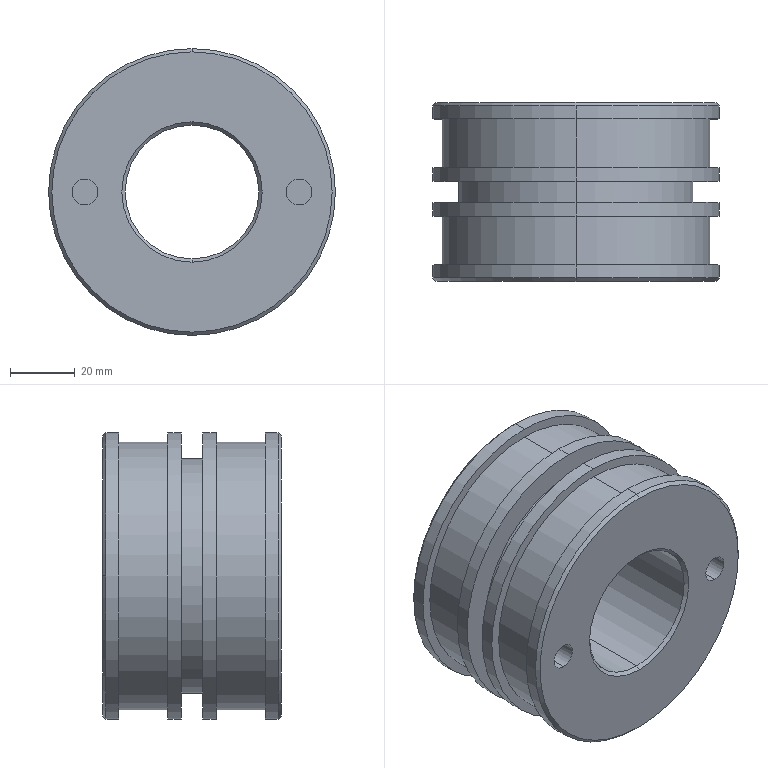Part | STEP file | 3. Piston | 1 solid | 41 faces | box 88.35 x 55 x 88.35 mm | volume 216858 mm3 | cylinder 22 | plane 11 | cone 8 | commonest cylinder face diameters 88.35 x8 8 x4 82.35 x4 41.25 x2 49 x2 72.35 x2
STEP:
#1=CARTESIAN_POINT('',(0.,40.,20.625));
#2=VERTEX_POINT('',#1);
#3=CARTESIAN_POINT('',(0.,40.,-20.625));
#4=VERTEX_POINT('',#3);
#5=CARTESIAN_POINT('',(0.,40.,0.));
#6=DIRECTION('',(0.,-1.,0.));
#7=DIRECTION('',(0.,0.,-1.));
#8=AXIS2_PLACEMENT_3D('',#5,#6,#7);
#9=CIRCLE('',#8,20.625);
#10=EDGE_CURVE('',#2,#4,#9,.T.);
#11=ORIENTED_EDGE('',*,*,#10,.F.);
#12=CARTESIAN_POINT('',(0.,1.,20.625));
#13=VERTEX_POINT('',#12);
#14=CARTESIAN_POINT('',(0.,55.,20.625));
#15=DIRECTION('',(0.,-1.,0.));
#16=VECTOR('',#15,1000.);
#17=LINE('',#14,#16);
#18=EDGE_CURVE('',#2,#13,#17,.T.);
#19=ORIENTED_EDGE('',*,*,#18,.T.);
#20=CARTESIAN_POINT('',(0.,1.,-20.625));
#21=VERTEX_POINT('',#20);
#22=CARTESIAN_POINT('',(0.,1.,0.));
#23=DIRECTION('',(0.,1.,0.));
#24=DIRECTION('',(0.,0.,-1.));
#25=AXIS2_PLACEMENT_3D('',#22,#23,#24);
#26=CIRCLE('',#25,20.625);
#27=EDGE_CURVE('',#21,#13,#26,.T.);
#28=ORIENTED_EDGE('',*,*,#27,.F.);
#29=CARTESIAN_POINT('',(0.,55.,-20.625));
#30=DIRECTION('',(0.,-1.,0.));
#31=VECTOR('',#30,1000.);
#32=LINE('',#29,#31);
#33=EDGE_CURVE('',#4,#21,#32,.T.);
#34=ORIENTED_EDGE('',*,*,#33,.F.);
#35=EDGE_LOOP('',(#11,#19,#28,#34));
#36=FACE_OUTER_BOUND('',#35,.T.);
#37=CARTESIAN_POINT('',(0.,55.,0.));
#38=DIRECTION('',(0.,-1.,0.));
#39=DIRECTION('',(0.,0.,-1.));
#40=AXIS2_PLACEMENT_3D('',#37,#38,#39);
#41=CYLINDRICAL_SURFACE('',#40,20.625);
#42=ADVANCED_FACE('',(#36),#41,.F.);
#43=ORIENTED_EDGE('',*,*,#27,.T.);
#44=CARTESIAN_POINT('',(0.,0.,21.625));
#45=VERTEX_POINT('',#44);
#46=CARTESIAN_POINT('',(0.,0.,21.625));
#47=DIRECTION('',(0.,-0.7071,0.7071));
#48=VECTOR('',#47,1000.);
#49=LINE('',#46,#48);
#50=EDGE_CURVE('',#13,#45,#49,.T.);
#51=ORIENTED_EDGE('',*,*,#50,.T.);
#52=CARTESIAN_POINT('',(0.,0.,-21.625));
#53=VERTEX_POINT('',#52);
#54=CARTESIAN_POINT('',(0.,0.,0.));
#55=DIRECTION('',(0.,1.,0.));
#56=DIRECTION('',(0.,0.,-1.));
#57=AXIS2_PLACEMENT_3D('',#54,#55,#56);
#58=CIRCLE('',#57,21.625);
#59=EDGE_CURVE('',#53,#45,#58,.T.);
#60=ORIENTED_EDGE('',*,*,#59,.F.);
#61=CARTESIAN_POINT('',(0.,0.,-21.625));
#62=DIRECTION('',(0.,-0.7071,-0.7071));
#63=VECTOR('',#62,1000.);
#64=LINE('',#61,#63);
#65=EDGE_CURVE('',#21,#53,#64,.T.);
#66=ORIENTED_EDGE('',*,*,#65,.F.);
#67=EDGE_LOOP('',(#43,#51,#60,#66));
#68=FACE_OUTER_BOUND('',#67,.T.);
#69=CARTESIAN_POINT('',(0.,0.,0.));
#70=DIRECTION('',(0.,-1.,0.));
#71=DIRECTION('',(0.,0.,-1.));
#72=AXIS2_PLACEMENT_3D('',#69,#70,#71);
#73=CONICAL_SURFACE('',#72,21.625,0.7854);
#74=ADVANCED_FACE('',(#68),#73,.F.);
#75=CARTESIAN_POINT('',(0.,40.,24.5));
#76=VERTEX_POINT('',#75);
#77=CARTESIAN_POINT('',(0.,40.,-24.5));
#78=VERTEX_POINT('',#77);
#79=CARTESIAN_POINT('',(0.,40.,0.));
#80=DIRECTION('',(0.,-1.,0.));
#81=DIRECTION('',(0.,0.,1.));
#82=AXIS2_PLACEMENT_3D('',#79,#80,#81);
#83=CIRCLE('',#82,24.5);
#84=EDGE_CURVE('',#76,#78,#83,.T.);
#85=ORIENTED_EDGE('',*,*,#84,.T.);
#86=CARTESIAN_POINT('',(0.,54.,-24.5));
#87=VERTEX_POINT('',#86);
#88=CARTESIAN_POINT('',(0.,40.,-24.5));
#89=DIRECTION('',(0.,1.,0.));
#90=VECTOR('',#89,1000.);
#91=LINE('',#88,#90);
#92=EDGE_CURVE('',#78,#87,#91,.T.);
#93=ORIENTED_EDGE('',*,*,#92,.T.);
#94=CARTESIAN_POINT('',(0.,54.,24.5));
#95=VERTEX_POINT('',#94);
#96=CARTESIAN_POINT('',(0.,54.,0.));
#97=DIRECTION('',(0.,-1.,0.));
#98=DIRECTION('',(0.,0.,1.));
#99=AXIS2_PLACEMENT_3D('',#96,#97,#98);
#100=CIRCLE('',#99,24.5);
#101=EDGE_CURVE('',#95,#87,#100,.T.);
#102=ORIENTED_EDGE('',*,*,#101,.F.);
#103=CARTESIAN_POINT('',(0.,40.,24.5));
#104=DIRECTION('',(0.,1.,0.));
#105=VECTOR('',#104,1000.);
#106=LINE('',#103,#105);
#107=EDGE_CURVE('',#76,#95,#106,.T.);
#108=ORIENTED_EDGE('',*,*,#107,.F.);
#109=EDGE_LOOP('',(#85,#93,#102,#108));
#110=FACE_OUTER_BOUND('',#109,.T.);
#111=CARTESIAN_POINT('',(0.,40.,0.));
#112=DIRECTION('',(0.,1.,0.));
#113=DIRECTION('',(0.,0.,1.));
#114=AXIS2_PLACEMENT_3D('',#111,#112,#113);
#115=CYLINDRICAL_SURFACE('',#114,24.5);
#116=ADVANCED_FACE('',(#110),#115,.F.);
#117=CARTESIAN_POINT('',(0.,0.,-43.175));
#118=VERTEX_POINT('',#117);
#119=CARTESIAN_POINT('',(0.,0.,43.175));
#120=VERTEX_POINT('',#119);
#121=CARTESIAN_POINT('',(0.,0.,0.));
#122=DIRECTION('',(0.,-1.,0.));
#123=DIRECTION('',(0.,0.,1.));
#124=AXIS2_PLACEMENT_3D('',#121,#122,#123);
#125=CIRCLE('',#124,43.175);
#126=EDGE_CURVE('',#118,#120,#125,.T.);
#127=ORIENTED_EDGE('',*,*,#126,.F.);
#128=CARTESIAN_POINT('',(0.,1.,-44.175));
#129=VERTEX_POINT('',#128);
#130=CARTESIAN_POINT('',(0.,1.,-44.175));
#131=DIRECTION('',(0.,0.7071,-0.7071));
#132=VECTOR('',#131,1000.);
#133=LINE('',#130,#132);
#134=EDGE_CURVE('',#118,#129,#133,.T.);
#135=ORIENTED_EDGE('',*,*,#134,.T.);
#136=CARTESIAN_POINT('',(0.,1.,44.175));
#137=VERTEX_POINT('',#136);
#138=CARTESIAN_POINT('',(0.,1.,0.));
#139=DIRECTION('',(0.,-1.,0.));
#140=DIRECTION('',(0.,0.,1.));
#141=AXIS2_PLACEMENT_3D('',#138,#139,#140);
#142=CIRCLE('',#141,44.175);
#143=EDGE_CURVE('',#129,#137,#142,.T.);
#144=ORIENTED_EDGE('',*,*,#143,.T.);
#145=CARTESIAN_POINT('',(0.,1.,44.175));
#146=DIRECTION('',(0.,0.7071,0.7071));
#147=VECTOR('',#146,1000.);
#148=LINE('',#145,#147);
#149=EDGE_CURVE('',#120,#137,#148,.T.);
#150=ORIENTED_EDGE('',*,*,#149,.F.);
#151=EDGE_LOOP('',(#127,#135,#144,#150));
#152=FACE_OUTER_BOUND('',#151,.T.);
#153=CARTESIAN_POINT('',(0.,1.,0.));
#154=DIRECTION('',(0.,1.,0.));
#155=DIRECTION('',(0.,0.,1.));
#156=AXIS2_PLACEMENT_3D('',#153,#154,#155);
#157=CONICAL_SURFACE('',#156,44.175,0.7854);
#158=ADVANCED_FACE('',(#152),#157,.T.);
#159=CARTESIAN_POINT('',(-33.,9.,4.));
#160=VERTEX_POINT('',#159);
#161=CARTESIAN_POINT('',(-33.,9.,-4.));
#162=VERTEX_POINT('',#161);
#163=CARTESIAN_POINT('',(-33.,9.,0.));
#164=DIRECTION('',(0.,-1.,0.));
#165=DIRECTION('',(0.,0.,-1.));
#166=AXIS2_PLACEMENT_3D('',#163,#164,#165);
#167=CIRCLE('',#166,4.);
#168=EDGE_CURVE('',#160,#162,#167,.T.);
#169=ORIENTED_EDGE('',*,*,#168,.F.);
#170=CARTESIAN_POINT('',(-33.,0.,4.));
#171=VERTEX_POINT('',#170);
#172=CARTESIAN_POINT('',(-33.,9.,4.));
#173=DIRECTION('',(0.,-1.,0.));
#174=VECTOR('',#173,1000.);
#175=LINE('',#172,#174);
#176=EDGE_CURVE('',#160,#171,#175,.T.);
#177=ORIENTED_EDGE('',*,*,#176,.T.);
#178=CARTESIAN_POINT('',(-33.,0.,-4.));
#179=VERTEX_POINT('',#178);
#180=CARTESIAN_POINT('',(-33.,0.,0.));
#181=DIRECTION('',(0.,1.,0.));
#182=DIRECTION('',(0.,0.,-1.));
#183=AXIS2_PLACEMENT_3D('',#180,#181,#182);
#184=CIRCLE('',#183,4.);
#185=EDGE_CURVE('',#179,#171,#184,.T.);
#186=ORIENTED_EDGE('',*,*,#185,.F.);
#187=CARTESIAN_POINT('',(-33.,9.,-4.));
#188=DIRECTION('',(0.,-1.,0.));
#189=VECTOR('',#188,1000.);
#190=LINE('',#187,#189);
#191=EDGE_CURVE('',#162,#179,#190,.T.);
#192=ORIENTED_EDGE('',*,*,#191,.F.);
#193=EDGE_LOOP('',(#169,#177,#186,#192));
#194=FACE_OUTER_BOUND('',#193,.T.);
#195=CARTESIAN_POINT('',(-33.,9.,0.));
#196=DIRECTION('',(0.,-1.,0.));
#197=DIRECTION('',(0.,0.,-1.));
#198=AXIS2_PLACEMENT_3D('',#195,#196,#197);
#199=CYLINDRICAL_SURFACE('',#198,4.);
#200=ADVANCED_FACE('',(#194),#199,.F.);
#201=CARTESIAN_POINT('',(33.,9.,4.));
#202=VERTEX_POINT('',#201);
#203=CARTESIAN_POINT('',(33.,9.,-4.));
#204=VERTEX_POINT('',#203);
#205=CARTESIAN_POINT('',(33.,9.,0.));
#206=DIRECTION('',(0.,-1.,0.));
#207=DIRECTION('',(0.,0.,-1.));
#208=AXIS2_PLACEMENT_3D('',#205,#206,#207);
#209=CIRCLE('',#208,4.);
#210=EDGE_CURVE('',#202,#204,#209,.T.);
#211=ORIENTED_EDGE('',*,*,#210,.F.);
#212=CARTESIAN_POINT('',(33.,0.,4.));
#213=VERTEX_POINT('',#212);
#214=CARTESIAN_POINT('',(33.,9.,4.));
#215=DIRECTION('',(0.,-1.,0.));
#216=VECTOR('',#215,1000.);
#217=LINE('',#214,#216);
#218=EDGE_CURVE('',#202,#213,#217,.T.);
#219=ORIENTED_EDGE('',*,*,#218,.T.);
#220=CARTESIAN_POINT('',(33.,0.,-4.));
#221=VERTEX_POINT('',#220);
#222=CARTESIAN_POINT('',(33.,0.,0.));
#223=DIRECTION('',(0.,1.,0.));
#224=DIRECTION('',(0.,0.,-1.));
#225=AXIS2_PLACEMENT_3D('',#222,#223,#224);
#226=CIRCLE('',#225,4.);
#227=EDGE_CURVE('',#221,#213,#226,.T.);
#228=ORIENTED_EDGE('',*,*,#227,.F.);
#229=CARTESIAN_POINT('',(33.,9.,-4.));
#230=DIRECTION('',(0.,-1.,0.));
#231=VECTOR('',#230,1000.);
#232=LINE('',#229,#231);
#233=EDGE_CURVE('',#204,#221,#232,.T.);
#234=ORIENTED_EDGE('',*,*,#233,.F.);
#235=EDGE_LOOP('',(#211,#219,#228,#234));
#236=FACE_OUTER_BOUND('',#235,.T.);
#237=CARTESIAN_POINT('',(33.,9.,0.));
#238=DIRECTION('',(0.,-1.,0.));
#239=DIRECTION('',(0.,0.,-1.));
#240=AXIS2_PLACEMENT_3D('',#237,#238,#239);
#241=CYLINDRICAL_SURFACE('',#240,4.);
#242=ADVANCED_FACE('',(#236),#241,.F.);
#243=ORIENTED_EDGE('',*,*,#101,.T.);
#244=CARTESIAN_POINT('',(0.,55.,-25.5));
#245=VERTEX_POINT('',#244);
#246=CARTESIAN_POINT('',(0.,55.,-25.5));
#247=DIRECTION('',(0.,0.7071,-0.7071));
#248=VECTOR('',#247,1000.);
#249=LINE('',#246,#248);
#250=EDGE_CURVE('',#87,#245,#249,.T.);
#251=ORIENTED_EDGE('',*,*,#250,.T.);
#252=CARTESIAN_POINT('',(0.,55.,25.5));
#253=VERTEX_POINT('',#252);
#254=CARTESIAN_POINT('',(0.,55.,0.));
#255=DIRECTION('',(0.,-1.,0.));
#256=DIRECTION('',(0.,0.,1.));
#257=AXIS2_PLACEMENT_3D('',#254,#255,#256);
#258=CIRCLE('',#257,25.5);
#259=EDGE_CURVE('',#253,#245,#258,.T.);
#260=ORIENTED_EDGE('',*,*,#259,.F.);
#261=CARTESIAN_POINT('',(0.,55.,25.5));
#262=DIRECTION('',(0.,0.7071,0.7071));
#263=VECTOR('',#262,1000.);
#264=LINE('',#261,#263);
#265=EDGE_CURVE('',#95,#253,#264,.T.);
#266=ORIENTED_EDGE('',*,*,#265,.F.);
#267=EDGE_LOOP('',(#243,#251,#260,#266));
#268=FACE_OUTER_BOUND('',#267,.T.);
#269=CARTESIAN_POINT('',(0.,55.,0.));
#270=DIRECTION('',(0.,1.,0.));
#271=DIRECTION('',(0.,0.,1.));
#272=AXIS2_PLACEMENT_3D('',#269,#270,#271);
#273=CONICAL_SURFACE('',#272,25.5,0.7854);
#274=ADVANCED_FACE('',(#268),#273,.F.);
#275=CARTESIAN_POINT('',(0.,5.,-44.175));
#276=VERTEX_POINT('',#275);
#277=CARTESIAN_POINT('',(0.,5.,44.175));
#278=VERTEX_POINT('',#277);
#279=CARTESIAN_POINT('',(0.,5.,0.));
#280=DIRECTION('',(0.,-1.,0.));
#281=DIRECTION('',(0.,0.,-1.));
#282=AXIS2_PLACEMENT_3D('',#279,#280,#281);
#283=CIRCLE('',#282,44.175);
#284=EDGE_CURVE('',#276,#278,#283,.T.);
#285=ORIENTED_EDGE('',*,*,#284,.T.);
#286=CARTESIAN_POINT('',(0.,55.,44.175));
#287=DIRECTION('',(0.,-1.,0.));
#288=VECTOR('',#287,1000.);
#289=LINE('',#286,#288);
#290=EDGE_CURVE('',#278,#137,#289,.T.);
#291=ORIENTED_EDGE('',*,*,#290,.T.);
#292=ORIENTED_EDGE('',*,*,#143,.F.);
#293=CARTESIAN_POINT('',(0.,55.,-44.175));
#294=DIRECTION('',(0.,-1.,0.));
#295=VECTOR('',#294,1000.);
#296=LINE('',#293,#295);
#297=EDGE_CURVE('',#276,#129,#296,.T.);
#298=ORIENTED_EDGE('',*,*,#297,.F.);
#299=EDGE_LOOP('',(#285,#291,#292,#298));
#300=FACE_OUTER_BOUND('',#299,.T.);
#301=CARTESIAN_POINT('',(0.,55.,0.));
#302=DIRECTION('',(0.,-1.,0.));
#303=DIRECTION('',(0.,0.,-1.));
#304=AXIS2_PLACEMENT_3D('',#301,#302,#303);
#305=CYLINDRICAL_SURFACE('',#304,44.175);
#306=ADVANCED_FACE('',(#300),#305,.T.);
#307=CARTESIAN_POINT('',(43.175,55.,0.));
#308=VERTEX_POINT('',#307);
#309=CARTESIAN_POINT('',(-43.175,55.,0.));
#310=VERTEX_POINT('',#309);
#311=CARTESIAN_POINT('',(0.,55.,0.));
#312=DIRECTION('',(0.,-1.,0.));
#313=DIRECTION('',(1.,0.,0.));
#314=AXIS2_PLACEMENT_3D('',#311,#312,#313);
#315=CIRCLE('',#314,43.175);
#316=EDGE_CURVE('',#308,#310,#315,.T.);
#317=ORIENTED_EDGE('',*,*,#316,.T.);
#318=CARTESIAN_POINT('',(-44.175,54.,0.));
#319=VERTEX_POINT('',#318);
#320=CARTESIAN_POINT('',(-44.175,54.,0.));
#321=DIRECTION('',(-0.7071,-0.7071,0.));
#322=VECTOR('',#321,1000.);
#323=LINE('',#320,#322);
#324=EDGE_CURVE('',#310,#319,#323,.T.);
#325=ORIENTED_EDGE('',*,*,#324,.T.);
#326=CARTESIAN_POINT('',(0.,54.,44.175));
#327=VERTEX_POINT('',#326);
#328=CARTESIAN_POINT('',(0.,54.,0.));
#329=DIRECTION('',(0.,1.,0.));
#330=DIRECTION('',(0.,0.,-1.));
#331=AXIS2_PLACEMENT_3D('',#328,#329,#330);
#332=CIRCLE('',#331,44.175);
#333=EDGE_CURVE('',#319,#327,#332,.T.);
#334=ORIENTED_EDGE('',*,*,#333,.T.);
#335=CARTESIAN_POINT('',(44.175,54.,0.));
#336=VERTEX_POINT('',#335);
#337=CARTESIAN_POINT('',(0.,54.,0.));
#338=DIRECTION('',(0.,1.,0.));
#339=DIRECTION('',(0.,0.,-1.));
#340=AXIS2_PLACEMENT_3D('',#337,#338,#339);
#341=CIRCLE('',#340,44.175);
#342=EDGE_CURVE('',#327,#336,#341,.T.);
#343=ORIENTED_EDGE('',*,*,#342,.T.);
#344=CARTESIAN_POINT('',(44.175,54.,0.));
#345=DIRECTION('',(0.7071,-0.7071,0.));
#346=VECTOR('',#345,1000.);
#347=LINE('',#344,#346);
#348=EDGE_CURVE('',#308,#336,#347,.T.);
#349=ORIENTED_EDGE('',*,*,#348,.F.);
#350=EDGE_LOOP('',(#317,#325,#334,#343,#349));
#351=FACE_OUTER_BOUND('',#350,.T.);
#352=CARTESIAN_POINT('',(0.,54.,0.));
#353=DIRECTION('',(0.,-1.,0.));
#354=DIRECTION('',(1.,0.,0.));
#355=AXIS2_PLACEMENT_3D('',#352,#353,#354);
#356=CONICAL_SURFACE('',#355,44.175,0.7854);
#357=ADVANCED_FACE('',(#351),#356,.T.);
#358=CARTESIAN_POINT('',(0.,20.,-41.175));
#359=VERTEX_POINT('',#358);
#360=CARTESIAN_POINT('',(0.,20.,41.175));
#361=VERTEX_POINT('',#360);
#362=CARTESIAN_POINT('',(0.,20.,0.));
#363=DIRECTION('',(0.,-1.,0.));
#364=DIRECTION('',(0.,0.,-1.));
#365=AXIS2_PLACEMENT_3D('',#362,#363,#364);
#366=CIRCLE('',#365,41.175);
#367=EDGE_CURVE('',#359,#361,#366,.T.);
#368=ORIENTED_EDGE('',*,*,#367,.T.);
#369=CARTESIAN_POINT('',(0.,5.,41.175));
#370=VERTEX_POINT('',#369);
#371=CARTESIAN_POINT('',(0.,1.1,41.175));
#372=DIRECTION('',(0.,-1.,0.));
#373=VECTOR('',#372,1000.);
#374=LINE('',#371,#373);
#375=EDGE_CURVE('',#361,#370,#374,.T.);
#376=ORIENTED_EDGE('',*,*,#375,.T.);
#377=CARTESIAN_POINT('',(0.,5.,-41.175));
#378=VERTEX_POINT('',#377);
#379=CARTESIAN_POINT('',(0.,5.,0.));
#380=DIRECTION('',(0.,-1.,0.));
#381=DIRECTION('',(0.,0.,-1.));
#382=AXIS2_PLACEMENT_3D('',#379,#380,#381);
#383=CIRCLE('',#382,41.175);
#384=EDGE_CURVE('',#378,#370,#383,.T.);
#385=ORIENTED_EDGE('',*,*,#384,.F.);
#386=CARTESIAN_POINT('',(0.,1.1,-41.175));
#387=DIRECTION('',(0.,-1.,0.));
#388=VECTOR('',#387,1000.);
#389=LINE('',#386,#388);
#390=EDGE_CURVE('',#359,#378,#389,.T.);
#391=ORIENTED_EDGE('',*,*,#390,.F.);
#392=EDGE_LOOP('',(#368,#376,#385,#391));
#393=FACE_OUTER_BOUND('',#392,.T.);
#394=CARTESIAN_POINT('',(0.,1.1,0.));
#395=DIRECTION('',(0.,-1.,0.));
#396=DIRECTION('',(0.,0.,-1.));
#397=AXIS2_PLACEMENT_3D('',#394,#395,#396);
#398=CYLINDRICAL_SURFACE('',#397,41.175);
#399=ADVANCED_FACE('',(#393),#398,.T.);
#400=ORIENTED_EDGE('',*,*,#342,.F.);
#401=CARTESIAN_POINT('',(0.,50.,44.175));
#402=VERTEX_POINT('',#401);
#403=CARTESIAN_POINT('',(0.,55.,44.175));
#404=DIRECTION('',(0.,-1.,0.));
#405=VECTOR('',#404,1000.);
#406=LINE('',#403,#405);
#407=EDGE_CURVE('',#327,#402,#406,.T.);
#408=ORIENTED_EDGE('',*,*,#407,.T.);
#409=CARTESIAN_POINT('',(0.,50.,-44.175));
#410=VERTEX_POINT('',#409);
#411=CARTESIAN_POINT('',(0.,50.,0.));
#412=DIRECTION('',(0.,1.,0.));
#413=DIRECTION('',(0.,0.,-1.));
#414=AXIS2_PLACEMENT_3D('',#411,#412,#413);
#415=CIRCLE('',#414,44.175);
#416=EDGE_CURVE('',#402,#410,#415,.T.);
#417=ORIENTED_EDGE('',*,*,#416,.T.);
#418=CARTESIAN_POINT('',(0.,54.,-44.175));
#419=VERTEX_POINT('',#418);
#420=CARTESIAN_POINT('',(0.,55.,-44.175));
#421=DIRECTION('',(0.,-1.,0.));
#422=VECTOR('',#421,1000.);
#423=LINE('',#420,#422);
#424=EDGE_CURVE('',#419,#410,#423,.T.);
#425=ORIENTED_EDGE('',*,*,#424,.F.);
#426=CARTESIAN_POINT('',(0.,54.,0.));
#427=DIRECTION('',(0.,1.,0.));
#428=DIRECTION('',(0.,0.,-1.));
#429=AXIS2_PLACEMENT_3D('',#426,#427,#428);
#430=CIRCLE('',#429,44.175);
#431=EDGE_CURVE('',#336,#419,#430,.T.);
#432=ORIENTED_EDGE('',*,*,#431,.F.);
#433=EDGE_LOOP('',(#400,#408,#417,#425,#432));
#434=FACE_OUTER_BOUND('',#433,.T.);
#435=CARTESIAN_POINT('',(0.,55.,0.));
#436=DIRECTION('',(0.,-1.,0.));
#437=DIRECTION('',(0.,0.,-1.));
#438=AXIS2_PLACEMENT_3D('',#435,#436,#437);
#439=CYLINDRICAL_SURFACE('',#438,44.175);
#440=ADVANCED_FACE('',(#434),#439,.T.);
#441=CARTESIAN_POINT('',(0.,24.25,-44.175));
#442=VERTEX_POINT('',#441);
#443=CARTESIAN_POINT('',(0.,24.25,44.175));
#444=VERTEX_POINT('',#443);
#445=CARTESIAN_POINT('',(0.,24.25,0.));
#446=DIRECTION('',(0.,-1.,0.));
#447=DIRECTION('',(0.,0.,-1.));
#448=AXIS2_PLACEMENT_3D('',#445,#446,#447);
#449=CIRCLE('',#448,44.175);
#450=EDGE_CURVE('',#442,#444,#449,.T.);
#451=ORIENTED_EDGE('',*,*,#450,.T.);
#452=CARTESIAN_POINT('',(0.,20.,44.175));
#453=VERTEX_POINT('',#452);
#454=CARTESIAN_POINT('',(0.,55.,44.175));
#455=DIRECTION('',(0.,-1.,0.));
#456=VECTOR('',#455,1000.);
#457=LINE('',#454,#456);
#458=EDGE_CURVE('',#444,#453,#457,.T.);
#459=ORIENTED_EDGE('',*,*,#458,.T.);
#460=CARTESIAN_POINT('',(0.,20.,-44.175));
#461=VERTEX_POINT('',#460);
#462=CARTESIAN_POINT('',(0.,20.,0.));
#463=DIRECTION('',(0.,-1.,0.));
#464=DIRECTION('',(0.,0.,-1.));
#465=AXIS2_PLACEMENT_3D('',#462,#463,#464);
#466=CIRCLE('',#465,44.175);
#467=EDGE_CURVE('',#461,#453,#466,.T.);
#468=ORIENTED_EDGE('',*,*,#467,.F.);
#469=CARTESIAN_POINT('',(0.,55.,-44.175));
#470=DIRECTION('',(0.,-1.,0.));
#471=VECTOR('',#470,1000.);
#472=LINE('',#469,#471);
#473=EDGE_CURVE('',#442,#461,#472,.T.);
#474=ORIENTED_EDGE('',*,*,#473,.F.);
#475=EDGE_LOOP('',(#451,#459,#468,#474));
#476=FACE_OUTER_BOUND('',#475,.T.);
#477=CARTESIAN_POINT('',(0.,55.,0.));
#478=DIRECTION('',(0.,-1.,0.));
#479=DIRECTION('',(0.,0.,-1.));
#480=AXIS2_PLACEMENT_3D('',#477,#478,#479);
#481=CYLINDRICAL_SURFACE('',#480,44.175);
#482=ADVANCED_FACE('',(#476),#481,.T.);
#483=CARTESIAN_POINT('',(0.,50.,41.175));
#484=VERTEX_POINT('',#483);
#485=CARTESIAN_POINT('',(0.,50.,-41.175));
#486=VERTEX_POINT('',#485);
#487=CARTESIAN_POINT('',(0.,50.,0.));
#488=DIRECTION('',(0.,1.,0.));
#489=DIRECTION('',(0.,0.,-1.));
#490=AXIS2_PLACEMENT_3D('',#487,#488,#489);
#491=CIRCLE('',#490,41.175);
#492=EDGE_CURVE('',#484,#486,#491,.T.);
#493=ORIENTED_EDGE('',*,*,#492,.F.);
#494=CARTESIAN_POINT('',(0.,35.,41.175));
#495=VERTEX_POINT('',#494);
#496=CARTESIAN_POINT('',(0.,1.1,41.175));
#497=DIRECTION('',(0.,-1.,0.));
#498=VECTOR('',#497,1000.);
#499=LINE('',#496,#498);
#500=EDGE_CURVE('',#484,#495,#499,.T.);
#501=ORIENTED_EDGE('',*,*,#500,.T.);
#502=CARTESIAN_POINT('',(0.,35.,-41.175));
#503=VERTEX_POINT('',#502);
#504=CARTESIAN_POINT('',(0.,35.,0.));
#505=DIRECTION('',(0.,1.,0.));
#506=DIRECTION('',(0.,0.,-1.));
#507=AXIS2_PLACEMENT_3D('',#504,#505,#506);
#508=CIRCLE('',#507,41.175);
#509=EDGE_CURVE('',#495,#503,#508,.T.);
#510=ORIENTED_EDGE('',*,*,#509,.T.);
#511=CARTESIAN_POINT('',(0.,1.1,-41.175));
#512=DIRECTION('',(0.,-1.,0.));
#513=VECTOR('',#512,1000.);
#514=LINE('',#511,#513);
#515=EDGE_CURVE('',#486,#503,#514,.T.);
#516=ORIENTED_EDGE('',*,*,#515,.F.);
#517=EDGE_LOOP('',(#493,#501,#510,#516));
#518=FACE_OUTER_BOUND('',#517,.T.);
#519=CARTESIAN_POINT('',(0.,1.1,0.));
#520=DIRECTION('',(0.,-1.,0.));
#521=DIRECTION('',(0.,0.,-1.));
#522=AXIS2_PLACEMENT_3D('',#519,#520,#521);
#523=CYLINDRICAL_SURFACE('',#522,41.175);
#524=ADVANCED_FACE('',(#518),#523,.T.);
#525=CARTESIAN_POINT('',(0.,30.75,-36.175));
#526=VERTEX_POINT('',#525);
#527=CARTESIAN_POINT('',(0.,30.75,36.175));
#528=VERTEX_POINT('',#527);
#529=CARTESIAN_POINT('',(0.,30.75,0.));
#530=DIRECTION('',(0.,-1.,0.));
#531=DIRECTION('',(0.,0.,-1.));
#532=AXIS2_PLACEMENT_3D('',#529,#530,#531);
#533=CIRCLE('',#532,36.175);
#534=EDGE_CURVE('',#526,#528,#533,.T.);
#535=ORIENTED_EDGE('',*,*,#534,.T.);
#536=CARTESIAN_POINT('',(0.,24.25,36.175));
#537=VERTEX_POINT('',#536);
#538=CARTESIAN_POINT('',(0.,1.1,36.175));
#539=DIRECTION('',(0.,-1.,0.));
#540=VECTOR('',#539,1000.);
#541=LINE('',#538,#540);
#542=EDGE_CURVE('',#528,#537,#541,.T.);
#543=ORIENTED_EDGE('',*,*,#542,.T.);
#544=CARTESIAN_POINT('',(0.,24.25,-36.175));
#545=VERTEX_POINT('',#544);
#546=CARTESIAN_POINT('',(0.,24.25,0.));
#547=DIRECTION('',(0.,-1.,0.));
#548=DIRECTION('',(0.,0.,-1.));
#549=AXIS2_PLACEMENT_3D('',#546,#547,#548);
#550=CIRCLE('',#549,36.175);
#551=EDGE_CURVE('',#545,#537,#550,.T.);
#552=ORIENTED_EDGE('',*,*,#551,.F.);
#553=CARTESIAN_POINT('',(0.,1.1,-36.175));
#554=DIRECTION('',(0.,-1.,0.));
#555=VECTOR('',#554,1000.);
#556=LINE('',#553,#555);
#557=EDGE_CURVE('',#526,#545,#556,.T.);
#558=ORIENTED_EDGE('',*,*,#557,.F.);
#559=EDGE_LOOP('',(#535,#543,#552,#558));
#560=FACE_OUTER_BOUND('',#559,.T.);
#561=CARTESIAN_POINT('',(0.,1.1,0.));
#562=DIRECTION('',(0.,-1.,0.));
#563=DIRECTION('',(0.,0.,-1.));
#564=AXIS2_PLACEMENT_3D('',#561,#562,#563);
#565=CYLINDRICAL_SURFACE('',#564,36.175);
#566=ADVANCED_FACE('',(#560),#565,.T.);
#567=CARTESIAN_POINT('',(0.,35.,44.175));
#568=VERTEX_POINT('',#567);
#569=CARTESIAN_POINT('',(0.,35.,-44.175));
#570=VERTEX_POINT('',#569);
#571=CARTESIAN_POINT('',(0.,35.,0.));
#572=DIRECTION('',(0.,1.,0.));
#573=DIRECTION('',(0.,0.,-1.));
#574=AXIS2_PLACEMENT_3D('',#571,#572,#573);
#575=CIRCLE('',#574,44.175);
#576=EDGE_CURVE('',#568,#570,#575,.T.);
#577=ORIENTED_EDGE('',*,*,#576,.F.);
#578=CARTESIAN_POINT('',(0.,30.75,44.175));
#579=VERTEX_POINT('',#578);
#580=CARTESIAN_POINT('',(0.,55.,44.175));
#581=DIRECTION('',(0.,-1.,0.));
#582=VECTOR('',#581,1000.);
#583=LINE('',#580,#582);
#584=EDGE_CURVE('',#568,#579,#583,.T.);
#585=ORIENTED_EDGE('',*,*,#584,.T.);
#586=CARTESIAN_POINT('',(0.,30.75,-44.175));
#587=VERTEX_POINT('',#586);
#588=CARTESIAN_POINT('',(0.,30.75,0.));
#589=DIRECTION('',(0.,1.,0.));
#590=DIRECTION('',(0.,0.,-1.));
#591=AXIS2_PLACEMENT_3D('',#588,#589,#590);
#592=CIRCLE('',#591,44.175);
#593=EDGE_CURVE('',#579,#587,#592,.T.);
#594=ORIENTED_EDGE('',*,*,#593,.T.);
#595=CARTESIAN_POINT('',(0.,55.,-44.175));
#596=DIRECTION('',(0.,-1.,0.));
#597=VECTOR('',#596,1000.);
#598=LINE('',#595,#597);
#599=EDGE_CURVE('',#570,#587,#598,.T.);
#600=ORIENTED_EDGE('',*,*,#599,.F.);
#601=EDGE_LOOP('',(#577,#585,#594,#600));
#602=FACE_OUTER_BOUND('',#601,.T.);
#603=CARTESIAN_POINT('',(0.,55.,0.));
#604=DIRECTION('',(0.,-1.,0.));
#605=DIRECTION('',(0.,0.,-1.));
#606=AXIS2_PLACEMENT_3D('',#603,#604,#605);
#607=CYLINDRICAL_SURFACE('',#606,44.175);
#608=ADVANCED_FACE('',(#602),#607,.T.);
#609=ORIENTED_EDGE('',*,*,#18,.F.);
#610=CARTESIAN_POINT('',(0.,40.,0.));
#611=DIRECTION('',(0.,-1.,0.));
#612=DIRECTION('',(0.,0.,-1.));
#613=AXIS2_PLACEMENT_3D('',#610,#611,#612);
#614=CIRCLE('',#613,20.625);
#615=EDGE_CURVE('',#4,#2,#614,.T.);
#616=ORIENTED_EDGE('',*,*,#615,.F.);
#617=ORIENTED_EDGE('',*,*,#33,.T.);
#618=CARTESIAN_POINT('',(0.,1.,0.));
#619=DIRECTION('',(0.,1.,0.));
#620=DIRECTION('',(0.,0.,-1.));
#621=AXIS2_PLACEMENT_3D('',#618,#619,#620);
#622=CIRCLE('',#621,20.625);
#623=EDGE_CURVE('',#13,#21,#622,.T.);
#624=ORIENTED_EDGE('',*,*,#623,.F.);
#625=EDGE_LOOP('',(#609,#616,#617,#624));
#626=FACE_OUTER_BOUND('',#625,.T.);
#627=CARTESIAN_POINT('',(0.,55.,0.));
#628=DIRECTION('',(0.,-1.,0.));
#629=DIRECTION('',(0.,0.,-1.));
#630=AXIS2_PLACEMENT_3D('',#627,#628,#629);
#631=CYLINDRICAL_SURFACE('',#630,20.625);
#632=ADVANCED_FACE('',(#626),#631,.F.);
#633=ORIENTED_EDGE('',*,*,#50,.F.);
#634=ORIENTED_EDGE('',*,*,#623,.T.);
#635=ORIENTED_EDGE('',*,*,#65,.T.);
#636=CARTESIAN_POINT('',(0.,0.,0.));
#637=DIRECTION('',(0.,1.,0.));
#638=DIRECTION('',(0.,0.,-1.));
#639=AXIS2_PLACEMENT_3D('',#636,#637,#638);
#640=CIRCLE('',#639,21.625);
#641=EDGE_CURVE('',#45,#53,#640,.T.);
#642=ORIENTED_EDGE('',*,*,#641,.F.);
#643=EDGE_LOOP('',(#633,#634,#635,#642));
#644=FACE_OUTER_BOUND('',#643,.T.);
#645=CARTESIAN_POINT('',(0.,0.,0.));
#646=DIRECTION('',(0.,-1.,0.));
#647=DIRECTION('',(0.,0.,-1.));
#648=AXIS2_PLACEMENT_3D('',#645,#646,#647);
#649=CONICAL_SURFACE('',#648,21.625,0.7854);
#650=ADVANCED_FACE('',(#644),#649,.F.);
#651=ORIENTED_EDGE('',*,*,#615,.T.);
#652=ORIENTED_EDGE('',*,*,#10,.T.);
#653=EDGE_LOOP('',(#651,#652));
#654=FACE_BOUND('',#653,.T.);
#655=ORIENTED_EDGE('',*,*,#84,.F.);
#656=CARTESIAN_POINT('',(0.,40.,0.));
#657=DIRECTION('',(0.,-1.,0.));
#658=DIRECTION('',(0.,0.,1.));
#659=AXIS2_PLACEMENT_3D('',#656,#657,#658);
#660=CIRCLE('',#659,24.5);
#661=EDGE_CURVE('',#78,#76,#660,.T.);
#662=ORIENTED_EDGE('',*,*,#661,.F.);
#663=EDGE_LOOP('',(#655,#662));
#664=FACE_OUTER_BOUND('',#663,.T.);
#665=CARTESIAN_POINT('',(0.,40.,0.));
#666=DIRECTION('',(0.,-1.,0.));
#667=DIRECTION('',(1.,0.,0.));
#668=AXIS2_PLACEMENT_3D('',#665,#666,#667);
#669=PLANE('',#668);
#670=ADVANCED_FACE('',(#654,#664),#669,.F.);
#671=ORIENTED_EDGE('',*,*,#59,.T.);
#672=ORIENTED_EDGE('',*,*,#641,.T.);
#673=EDGE_LOOP('',(#671,#672));
#674=FACE_BOUND('',#673,.T.);
#675=CARTESIAN_POINT('',(0.,0.,0.));
#676=DIRECTION('',(0.,-1.,0.));
#677=DIRECTION('',(0.,0.,1.));
#678=AXIS2_PLACEMENT_3D('',#675,#676,#677);
#679=CIRCLE('',#678,43.175);
#680=EDGE_CURVE('',#120,#118,#679,.T.);
#681=ORIENTED_EDGE('',*,*,#680,.T.);
#682=ORIENTED_EDGE('',*,*,#126,.T.);
#683=EDGE_LOOP('',(#681,#682));
#684=FACE_OUTER_BOUND('',#683,.T.);
#685=ORIENTED_EDGE('',*,*,#185,.T.);
#686=CARTESIAN_POINT('',(-33.,0.,0.));
#687=DIRECTION('',(0.,1.,0.));
#688=DIRECTION('',(0.,0.,-1.));
#689=AXIS2_PLACEMENT_3D('',#686,#687,#688);
#690=CIRCLE('',#689,4.);
#691=EDGE_CURVE('',#171,#179,#690,.T.);
#692=ORIENTED_EDGE('',*,*,#691,.T.);
#693=EDGE_LOOP('',(#685,#692));
#694=FACE_BOUND('',#693,.T.);
#695=ORIENTED_EDGE('',*,*,#227,.T.);
#696=CARTESIAN_POINT('',(33.,0.,0.));
#697=DIRECTION('',(0.,1.,0.));
#698=DIRECTION('',(0.,0.,-1.));
#699=AXIS2_PLACEMENT_3D('',#696,#697,#698);
#700=CIRCLE('',#699,4.);
#701=EDGE_CURVE('',#213,#221,#700,.T.);
#702=ORIENTED_EDGE('',*,*,#701,.T.);
#703=EDGE_LOOP('',(#695,#702));
#704=FACE_BOUND('',#703,.T.);
#705=CARTESIAN_POINT('',(0.,0.,0.));
#706=DIRECTION('',(0.,-1.,0.));
#707=DIRECTION('',(0.,0.,-1.));
#708=AXIS2_PLACEMENT_3D('',#705,#706,#707);
#709=PLANE('',#708);
#710=ADVANCED_FACE('',(#674,#684,#694,#704),#709,.T.);
#711=ORIENTED_EDGE('',*,*,#92,.F.);
#712=ORIENTED_EDGE('',*,*,#661,.T.);
#713=ORIENTED_EDGE('',*,*,#107,.T.);
#714=CARTESIAN_POINT('',(0.,54.,0.));
#715=DIRECTION('',(0.,-1.,0.));
#716=DIRECTION('',(0.,0.,1.));
#717=AXIS2_PLACEMENT_3D('',#714,#715,#716);
#718=CIRCLE('',#717,24.5);
#719=EDGE_CURVE('',#87,#95,#718,.T.);
#720=ORIENTED_EDGE('',*,*,#719,.F.);
#721=EDGE_LOOP('',(#711,#712,#713,#720));
#722=FACE_OUTER_BOUND('',#721,.T.);
#723=CARTESIAN_POINT('',(0.,40.,0.));
#724=DIRECTION('',(0.,1.,0.));
#725=DIRECTION('',(0.,0.,1.));
#726=AXIS2_PLACEMENT_3D('',#723,#724,#725);
#727=CYLINDRICAL_SURFACE('',#726,24.5);
#728=ADVANCED_FACE('',(#722),#727,.F.);
#729=ORIENTED_EDGE('',*,*,#134,.F.);
#730=ORIENTED_EDGE('',*,*,#680,.F.);
#731=ORIENTED_EDGE('',*,*,#149,.T.);
#732=CARTESIAN_POINT('',(0.,1.,0.));
#733=DIRECTION('',(0.,-1.,0.));
#734=DIRECTION('',(0.,0.,1.));
#735=AXIS2_PLACEMENT_3D('',#732,#733,#734);
#736=CIRCLE('',#735,44.175);
#737=EDGE_CURVE('',#137,#129,#736,.T.);
#738=ORIENTED_EDGE('',*,*,#737,.T.);
#739=EDGE_LOOP('',(#729,#730,#731,#738));
#740=FACE_OUTER_BOUND('',#739,.T.);
#741=CARTESIAN_POINT('',(0.,1.,0.));
#742=DIRECTION('',(0.,1.,0.));
#743=DIRECTION('',(0.,0.,1.));
#744=AXIS2_PLACEMENT_3D('',#741,#742,#743);
#745=CONICAL_SURFACE('',#744,44.175,0.7854);
#746=ADVANCED_FACE('',(#740),#745,.T.);
#747=ORIENTED_EDGE('',*,*,#176,.F.);
#748=CARTESIAN_POINT('',(-33.,9.,0.));
#749=DIRECTION('',(0.,-1.,0.));
#750=DIRECTION('',(0.,0.,-1.));
#751=AXIS2_PLACEMENT_3D('',#748,#749,#750);
#752=CIRCLE('',#751,4.);
#753=EDGE_CURVE('',#162,#160,#752,.T.);
#754=ORIENTED_EDGE('',*,*,#753,.F.);
#755=ORIENTED_EDGE('',*,*,#191,.T.);
#756=ORIENTED_EDGE('',*,*,#691,.F.);
#757=EDGE_LOOP('',(#747,#754,#755,#756));
#758=FACE_OUTER_BOUND('',#757,.T.);
#759=CARTESIAN_POINT('',(-33.,9.,0.));
#760=DIRECTION('',(0.,-1.,0.));
#761=DIRECTION('',(0.,0.,-1.));
#762=AXIS2_PLACEMENT_3D('',#759,#760,#761);
#763=CYLINDRICAL_SURFACE('',#762,4.);
#764=ADVANCED_FACE('',(#758),#763,.F.);
#765=ORIENTED_EDGE('',*,*,#218,.F.);
#766=CARTESIAN_POINT('',(33.,9.,0.));
#767=DIRECTION('',(0.,-1.,0.));
#768=DIRECTION('',(0.,0.,-1.));
#769=AXIS2_PLACEMENT_3D('',#766,#767,#768);
#770=CIRCLE('',#769,4.);
#771=EDGE_CURVE('',#204,#202,#770,.T.);
#772=ORIENTED_EDGE('',*,*,#771,.F.);
#773=ORIENTED_EDGE('',*,*,#233,.T.);
#774=ORIENTED_EDGE('',*,*,#701,.F.);
#775=EDGE_LOOP('',(#765,#772,#773,#774));
#776=FACE_OUTER_BOUND('',#775,.T.);
#777=CARTESIAN_POINT('',(33.,9.,0.));
#778=DIRECTION('',(0.,-1.,0.));
#779=DIRECTION('',(0.,0.,-1.));
#780=AXIS2_PLACEMENT_3D('',#777,#778,#779);
#781=CYLINDRICAL_SURFACE('',#780,4.);
#782=ADVANCED_FACE('',(#776),#781,.F.);
#783=ORIENTED_EDGE('',*,*,#250,.F.);
#784=ORIENTED_EDGE('',*,*,#719,.T.);
#785=ORIENTED_EDGE('',*,*,#265,.T.);
#786=CARTESIAN_POINT('',(0.,55.,0.));
#787=DIRECTION('',(0.,-1.,0.));
#788=DIRECTION('',(0.,0.,1.));
#789=AXIS2_PLACEMENT_3D('',#786,#787,#788);
#790=CIRCLE('',#789,25.5);
#791=EDGE_CURVE('',#245,#253,#790,.T.);
#792=ORIENTED_EDGE('',*,*,#791,.F.);
#793=EDGE_LOOP('',(#783,#784,#785,#792));
#794=FACE_OUTER_BOUND('',#793,.T.);
#795=CARTESIAN_POINT('',(0.,55.,0.));
#796=DIRECTION('',(0.,1.,0.));
#797=DIRECTION('',(0.,0.,1.));
#798=AXIS2_PLACEMENT_3D('',#795,#796,#797);
#799=CONICAL_SURFACE('',#798,25.5,0.7854);
#800=ADVANCED_FACE('',(#794),#799,.F.);
#801=ORIENTED_EDGE('',*,*,#290,.F.);
#802=CARTESIAN_POINT('',(0.,5.,0.));
#803=DIRECTION('',(0.,-1.,0.));
#804=DIRECTION('',(0.,0.,-1.));
#805=AXIS2_PLACEMENT_3D('',#802,#803,#804);
#806=CIRCLE('',#805,44.175);
#807=EDGE_CURVE('',#278,#276,#806,.T.);
#808=ORIENTED_EDGE('',*,*,#807,.T.);
#809=ORIENTED_EDGE('',*,*,#297,.T.);
#810=ORIENTED_EDGE('',*,*,#737,.F.);
#811=EDGE_LOOP('',(#801,#808,#809,#810));
#812=FACE_OUTER_BOUND('',#811,.T.);
#813=CARTESIAN_POINT('',(0.,55.,0.));
#814=DIRECTION('',(0.,-1.,0.));
#815=DIRECTION('',(0.,0.,-1.));
#816=AXIS2_PLACEMENT_3D('',#813,#814,#815);
#817=CYLINDRICAL_SURFACE('',#816,44.175);
#818=ADVANCED_FACE('',(#812),#817,.T.);
#819=ORIENTED_EDGE('',*,*,#753,.T.);
#820=ORIENTED_EDGE('',*,*,#168,.T.);
#821=EDGE_LOOP('',(#819,#820));
#822=FACE_OUTER_BOUND('',#821,.T.);
#823=CARTESIAN_POINT('',(-33.,9.,0.));
#824=DIRECTION('',(0.,1.,0.));
#825=DIRECTION('',(0.,0.,1.));
#826=AXIS2_PLACEMENT_3D('',#823,#824,#825);
#827=PLANE('',#826);
#828=ADVANCED_FACE('',(#822),#827,.F.);
#829=ORIENTED_EDGE('',*,*,#771,.T.);
#830=ORIENTED_EDGE('',*,*,#210,.T.);
#831=EDGE_LOOP('',(#829,#830));
#832=FACE_OUTER_BOUND('',#831,.T.);
#833=CARTESIAN_POINT('',(33.,9.,0.));
#834=DIRECTION('',(0.,1.,0.));
#835=DIRECTION('',(0.,0.,1.));
#836=AXIS2_PLACEMENT_3D('',#833,#834,#835);
#837=PLANE('',#836);
#838=ADVANCED_FACE('',(#832),#837,.F.);
#839=ORIENTED_EDGE('',*,*,#316,.F.);
#840=CARTESIAN_POINT('',(0.,55.,0.));
#841=DIRECTION('',(0.,-1.,0.));
#842=DIRECTION('',(1.,0.,0.));
#843=AXIS2_PLACEMENT_3D('',#840,#841,#842);
#844=CIRCLE('',#843,43.175);
#845=EDGE_CURVE('',#310,#308,#844,.T.);
#846=ORIENTED_EDGE('',*,*,#845,.F.);
#847=EDGE_LOOP('',(#839,#846));
#848=FACE_OUTER_BOUND('',#847,.T.);
#849=ORIENTED_EDGE('',*,*,#259,.T.);
#850=ORIENTED_EDGE('',*,*,#791,.T.);
#851=EDGE_LOOP('',(#849,#850));
#852=FACE_BOUND('',#851,.T.);
#853=CARTESIAN_POINT('',(0.,55.,0.));
#854=DIRECTION('',(0.,-1.,0.));
#855=DIRECTION('',(0.,0.,-1.));
#856=AXIS2_PLACEMENT_3D('',#853,#854,#855);
#857=PLANE('',#856);
#858=ADVANCED_FACE('',(#848,#852),#857,.F.);
#859=ORIENTED_EDGE('',*,*,#284,.F.);
#860=ORIENTED_EDGE('',*,*,#807,.F.);
#861=EDGE_LOOP('',(#859,#860));
#862=FACE_OUTER_BOUND('',#861,.T.);
#863=ORIENTED_EDGE('',*,*,#384,.T.);
#864=CARTESIAN_POINT('',(0.,5.,0.));
#865=DIRECTION('',(0.,-1.,0.));
#866=DIRECTION('',(0.,0.,-1.));
#867=AXIS2_PLACEMENT_3D('',#864,#865,#866);
#868=CIRCLE('',#867,41.175);
#869=EDGE_CURVE('',#370,#378,#868,.T.);
#870=ORIENTED_EDGE('',*,*,#869,.T.);
#871=EDGE_LOOP('',(#863,#870));
#872=FACE_BOUND('',#871,.T.);
#873=CARTESIAN_POINT('',(0.,5.,-44.175));
#874=DIRECTION('',(0.,1.,0.));
#875=DIRECTION('',(0.,0.,1.));
#876=AXIS2_PLACEMENT_3D('',#873,#874,#875);
#877=PLANE('',#876);
#878=ADVANCED_FACE('',(#862,#872),#877,.T.);
#879=ORIENTED_EDGE('',*,*,#324,.F.);
#880=ORIENTED_EDGE('',*,*,#845,.T.);
#881=ORIENTED_EDGE('',*,*,#348,.T.);
#882=ORIENTED_EDGE('',*,*,#431,.T.);
#883=CARTESIAN_POINT('',(0.,54.,0.));
#884=DIRECTION('',(0.,1.,0.));
#885=DIRECTION('',(0.,0.,-1.));
#886=AXIS2_PLACEMENT_3D('',#883,#884,#885);
#887=CIRCLE('',#886,44.175);
#888=EDGE_CURVE('',#419,#319,#887,.T.);
#889=ORIENTED_EDGE('',*,*,#888,.T.);
#890=EDGE_LOOP('',(#879,#880,#881,#882,#889));
#891=FACE_OUTER_BOUND('',#890,.T.);
#892=CARTESIAN_POINT('',(0.,54.,0.));
#893=DIRECTION('',(0.,-1.,0.));
#894=DIRECTION('',(1.,0.,0.));
#895=AXIS2_PLACEMENT_3D('',#892,#893,#894);
#896=CONICAL_SURFACE('',#895,44.175,0.7854);
#897=ADVANCED_FACE('',(#891),#896,.T.);
#898=ORIENTED_EDGE('',*,*,#375,.F.);
#899=CARTESIAN_POINT('',(0.,20.,0.));
#900=DIRECTION('',(0.,-1.,0.));
#901=DIRECTION('',(0.,0.,-1.));
#902=AXIS2_PLACEMENT_3D('',#899,#900,#901);
#903=CIRCLE('',#902,41.175);
#904=EDGE_CURVE('',#361,#359,#903,.T.);
#905=ORIENTED_EDGE('',*,*,#904,.T.);
#906=ORIENTED_EDGE('',*,*,#390,.T.);
#907=ORIENTED_EDGE('',*,*,#869,.F.);
#908=EDGE_LOOP('',(#898,#905,#906,#907));
#909=FACE_OUTER_BOUND('',#908,.T.);
#910=CARTESIAN_POINT('',(0.,1.1,0.));
#911=DIRECTION('',(0.,-1.,0.));
#912=DIRECTION('',(0.,0.,-1.));
#913=AXIS2_PLACEMENT_3D('',#910,#911,#912);
#914=CYLINDRICAL_SURFACE('',#913,41.175);
#915=ADVANCED_FACE('',(#909),#914,.T.);
#916=ORIENTED_EDGE('',*,*,#407,.F.);
#917=ORIENTED_EDGE('',*,*,#333,.F.);
#918=ORIENTED_EDGE('',*,*,#888,.F.);
#919=ORIENTED_EDGE('',*,*,#424,.T.);
#920=CARTESIAN_POINT('',(0.,50.,0.));
#921=DIRECTION('',(0.,1.,0.));
#922=DIRECTION('',(0.,0.,-1.));
#923=AXIS2_PLACEMENT_3D('',#920,#921,#922);
#924=CIRCLE('',#923,44.175);
#925=EDGE_CURVE('',#410,#402,#924,.T.);
#926=ORIENTED_EDGE('',*,*,#925,.T.);
#927=EDGE_LOOP('',(#916,#917,#918,#919,#926));
#928=FACE_OUTER_BOUND('',#927,.T.);
#929=CARTESIAN_POINT('',(0.,55.,0.));
#930=DIRECTION('',(0.,-1.,0.));
#931=DIRECTION('',(0.,0.,-1.));
#932=AXIS2_PLACEMENT_3D('',#929,#930,#931);
#933=CYLINDRICAL_SURFACE('',#932,44.175);
#934=ADVANCED_FACE('',(#928),#933,.T.);
#935=ORIENTED_EDGE('',*,*,#367,.F.);
#936=ORIENTED_EDGE('',*,*,#904,.F.);
#937=EDGE_LOOP('',(#935,#936));
#938=FACE_BOUND('',#937,.T.);
#939=ORIENTED_EDGE('',*,*,#467,.T.);
#940=CARTESIAN_POINT('',(0.,20.,0.));
#941=DIRECTION('',(0.,-1.,0.));
#942=DIRECTION('',(0.,0.,-1.));
#943=AXIS2_PLACEMENT_3D('',#940,#941,#942);
#944=CIRCLE('',#943,44.175);
#945=EDGE_CURVE('',#453,#461,#944,.T.);
#946=ORIENTED_EDGE('',*,*,#945,.T.);
#947=EDGE_LOOP('',(#939,#946));
#948=FACE_OUTER_BOUND('',#947,.T.);
#949=CARTESIAN_POINT('',(0.,20.,-41.175));
#950=DIRECTION('',(0.,-1.,0.));
#951=DIRECTION('',(0.,0.,-1.));
#952=AXIS2_PLACEMENT_3D('',#949,#950,#951);
#953=PLANE('',#952);
#954=ADVANCED_FACE('',(#938,#948),#953,.T.);
#955=CARTESIAN_POINT('',(0.,50.,0.));
#956=DIRECTION('',(0.,1.,0.));
#957=DIRECTION('',(0.,0.,-1.));
#958=AXIS2_PLACEMENT_3D('',#955,#956,#957);
#959=CIRCLE('',#958,41.175);
#960=EDGE_CURVE('',#486,#484,#959,.T.);
#961=ORIENTED_EDGE('',*,*,#960,.T.);
#962=ORIENTED_EDGE('',*,*,#492,.T.);
#963=EDGE_LOOP('',(#961,#962));
#964=FACE_BOUND('',#963,.T.);
#965=ORIENTED_EDGE('',*,*,#925,.F.);
#966=ORIENTED_EDGE('',*,*,#416,.F.);
#967=EDGE_LOOP('',(#965,#966));
#968=FACE_OUTER_BOUND('',#967,.T.);
#969=CARTESIAN_POINT('',(0.,50.,-41.175));
#970=DIRECTION('',(0.,-1.,0.));
#971=DIRECTION('',(0.,0.,-1.));
#972=AXIS2_PLACEMENT_3D('',#969,#970,#971);
#973=PLANE('',#972);
#974=ADVANCED_FACE('',(#964,#968),#973,.T.);
#975=ORIENTED_EDGE('',*,*,#458,.F.);
#976=CARTESIAN_POINT('',(0.,24.25,0.));
#977=DIRECTION('',(0.,-1.,0.));
#978=DIRECTION('',(0.,0.,-1.));
#979=AXIS2_PLACEMENT_3D('',#976,#977,#978);
#980=CIRCLE('',#979,44.175);
#981=EDGE_CURVE('',#444,#442,#980,.T.);
#982=ORIENTED_EDGE('',*,*,#981,.T.);
#983=ORIENTED_EDGE('',*,*,#473,.T.);
#984=ORIENTED_EDGE('',*,*,#945,.F.);
#985=EDGE_LOOP('',(#975,#982,#983,#984));
#986=FACE_OUTER_BOUND('',#985,.T.);
#987=CARTESIAN_POINT('',(0.,55.,0.));
#988=DIRECTION('',(0.,-1.,0.));
#989=DIRECTION('',(0.,0.,-1.));
#990=AXIS2_PLACEMENT_3D('',#987,#988,#989);
#991=CYLINDRICAL_SURFACE('',#990,44.175);
#992=ADVANCED_FACE('',(#986),#991,.T.);
#993=ORIENTED_EDGE('',*,*,#500,.F.);
#994=ORIENTED_EDGE('',*,*,#960,.F.);
#995=ORIENTED_EDGE('',*,*,#515,.T.);
#996=CARTESIAN_POINT('',(0.,35.,0.));
#997=DIRECTION('',(0.,1.,0.));
#998=DIRECTION('',(0.,0.,-1.));
#999=AXIS2_PLACEMENT_3D('',#996,#997,#998);
#1000=CIRCLE('',#999,41.175);
#1001=EDGE_CURVE('',#503,#495,#1000,.T.);
#1002=ORIENTED_EDGE('',*,*,#1001,.T.);
#1003=EDGE_LOOP('',(#993,#994,#995,#1002));
#1004=FACE_OUTER_BOUND('',#1003,.T.);
#1005=CARTESIAN_POINT('',(0.,1.1,0.));
#1006=DIRECTION('',(0.,-1.,0.));
#1007=DIRECTION('',(0.,0.,-1.));
#1008=AXIS2_PLACEMENT_3D('',#1005,#1006,#1007);
#1009=CYLINDRICAL_SURFACE('',#1008,41.175);
#1010=ADVANCED_FACE('',(#1004),#1009,.T.);
#1011=ORIENTED_EDGE('',*,*,#450,.F.);
#1012=ORIENTED_EDGE('',*,*,#981,.F.);
#1013=EDGE_LOOP('',(#1011,#1012));
#1014=FACE_OUTER_BOUND('',#1013,.T.);
#1015=ORIENTED_EDGE('',*,*,#551,.T.);
#1016=CARTESIAN_POINT('',(0.,24.25,0.));
#1017=DIRECTION('',(0.,-1.,0.));
#1018=DIRECTION('',(0.,0.,-1.));
#1019=AXIS2_PLACEMENT_3D('',#1016,#1017,#1018);
#1020=CIRCLE('',#1019,36.175);
#1021=EDGE_CURVE('',#537,#545,#1020,.T.);
#1022=ORIENTED_EDGE('',*,*,#1021,.T.);
#1023=EDGE_LOOP('',(#1015,#1022));
#1024=FACE_BOUND('',#1023,.T.);
#1025=CARTESIAN_POINT('',(0.,24.25,-44.175));
#1026=DIRECTION('',(0.,1.,0.));
#1027=DIRECTION('',(0.,0.,1.));
#1028=AXIS2_PLACEMENT_3D('',#1025,#1026,#1027);
#1029=PLANE('',#1028);
#1030=ADVANCED_FACE('',(#1014,#1024),#1029,.T.);
#1031=CARTESIAN_POINT('',(0.,35.,0.));
#1032=DIRECTION('',(0.,1.,0.));
#1033=DIRECTION('',(0.,0.,-1.));
#1034=AXIS2_PLACEMENT_3D('',#1031,#1032,#1033);
#1035=CIRCLE('',#1034,44.175);
#1036=EDGE_CURVE('',#570,#568,#1035,.T.);
#1037=ORIENTED_EDGE('',*,*,#1036,.T.);
#1038=ORIENTED_EDGE('',*,*,#576,.T.);
#1039=EDGE_LOOP('',(#1037,#1038));
#1040=FACE_OUTER_BOUND('',#1039,.T.);
#1041=ORIENTED_EDGE('',*,*,#1001,.F.);
#1042=ORIENTED_EDGE('',*,*,#509,.F.);
#1043=EDGE_LOOP('',(#1041,#1042));
#1044=FACE_BOUND('',#1043,.T.);
#1045=CARTESIAN_POINT('',(0.,35.,-44.175));
#1046=DIRECTION('',(0.,1.,0.));
#1047=DIRECTION('',(0.,0.,1.));
#1048=AXIS2_PLACEMENT_3D('',#1045,#1046,#1047);
#1049=PLANE('',#1048);
#1050=ADVANCED_FACE('',(#1040,#1044),#1049,.T.);
#1051=ORIENTED_EDGE('',*,*,#542,.F.);
#1052=CARTESIAN_POINT('',(0.,30.75,0.));
#1053=DIRECTION('',(0.,-1.,0.));
#1054=DIRECTION('',(0.,0.,-1.));
#1055=AXIS2_PLACEMENT_3D('',#1052,#1053,#1054);
#1056=CIRCLE('',#1055,36.175);
#1057=EDGE_CURVE('',#528,#526,#1056,.T.);
#1058=ORIENTED_EDGE('',*,*,#1057,.T.);
#1059=ORIENTED_EDGE('',*,*,#557,.T.);
#1060=ORIENTED_EDGE('',*,*,#1021,.F.);
#1061=EDGE_LOOP('',(#1051,#1058,#1059,#1060));
#1062=FACE_OUTER_BOUND('',#1061,.T.);
#1063=CARTESIAN_POINT('',(0.,1.1,0.));
#1064=DIRECTION('',(0.,-1.,0.));
#1065=DIRECTION('',(0.,0.,-1.));
#1066=AXIS2_PLACEMENT_3D('',#1063,#1064,#1065);
#1067=CYLINDRICAL_SURFACE('',#1066,36.175);
#1068=ADVANCED_FACE('',(#1062),#1067,.T.);
#1069=ORIENTED_EDGE('',*,*,#584,.F.);
#1070=ORIENTED_EDGE('',*,*,#1036,.F.);
#1071=ORIENTED_EDGE('',*,*,#599,.T.);
#1072=CARTESIAN_POINT('',(0.,30.75,0.));
#1073=DIRECTION('',(0.,1.,0.));
#1074=DIRECTION('',(0.,0.,-1.));
#1075=AXIS2_PLACEMENT_3D('',#1072,#1073,#1074);
#1076=CIRCLE('',#1075,44.175);
#1077=EDGE_CURVE('',#587,#579,#1076,.T.);
#1078=ORIENTED_EDGE('',*,*,#1077,.T.);
#1079=EDGE_LOOP('',(#1069,#1070,#1071,#1078));
#1080=FACE_OUTER_BOUND('',#1079,.T.);
#1081=CARTESIAN_POINT('',(0.,55.,0.));
#1082=DIRECTION('',(0.,-1.,0.));
#1083=DIRECTION('',(0.,0.,-1.));
#1084=AXIS2_PLACEMENT_3D('',#1081,#1082,#1083);
#1085=CYLINDRICAL_SURFACE('',#1084,44.175);
#1086=ADVANCED_FACE('',(#1080),#1085,.T.);
#1087=ORIENTED_EDGE('',*,*,#534,.F.);
#1088=ORIENTED_EDGE('',*,*,#1057,.F.);
#1089=EDGE_LOOP('',(#1087,#1088));
#1090=FACE_BOUND('',#1089,.T.);
#1091=ORIENTED_EDGE('',*,*,#1077,.F.);
#1092=ORIENTED_EDGE('',*,*,#593,.F.);
#1093=EDGE_LOOP('',(#1091,#1092));
#1094=FACE_OUTER_BOUND('',#1093,.T.);
#1095=CARTESIAN_POINT('',(0.,30.75,-36.175));
#1096=DIRECTION('',(0.,-1.,0.));
#1097=DIRECTION('',(0.,0.,-1.));
#1098=AXIS2_PLACEMENT_3D('',#1095,#1096,#1097);
#1099=PLANE('',#1098);
#1100=ADVANCED_FACE('',(#1090,#1094),#1099,.T.);
#1101=CLOSED_SHELL('',(#42,#74,#116,#158,#200,#242,#274,#306,#357,#399,#440,#482,#524,#566,#608,#632,#650,#670,#710,#728,#746,#764,#782,#800,#818,#828,#838,#858,#878,#897,#915,#934,#954,#974,#992,#1010,#1030,#1050,#1068,#1086,#1100));
#1102=MANIFOLD_SOLID_BREP('',#1101);
#1103=CARTESIAN_POINT('',(0.,0.,0.));
#1104=DIRECTION('',(0.,0.,1.));
#1105=DIRECTION('',(1.,0.,0.));
#1106=AXIS2_PLACEMENT_3D('',#1103,#1104,#1105);
#1107=(LENGTH_UNIT()NAMED_UNIT(*)SI_UNIT(.MILLI.,.METRE.));
#1108=UNCERTAINTY_MEASURE_WITH_UNIT(LENGTH_MEASURE(0.00001),#1107,'','');
#1109=(NAMED_UNIT(*)PLANE_ANGLE_UNIT()SI_UNIT($,.RADIAN.));
#1110=(NAMED_UNIT(*)SI_UNIT($,.STERADIAN.)SOLID_ANGLE_UNIT());
#1111=(GEOMETRIC_REPRESENTATION_CONTEXT(3)GLOBAL_UNCERTAINTY_ASSIGNED_CONTEXT((#1108))GLOBAL_UNIT_ASSIGNED_CONTEXT((#1107,#1109,#1110))REPRESENTATION_CONTEXT('',''));
#1112=ADVANCED_BREP_SHAPE_REPRESENTATION('',(#1102,#1106),#1111);